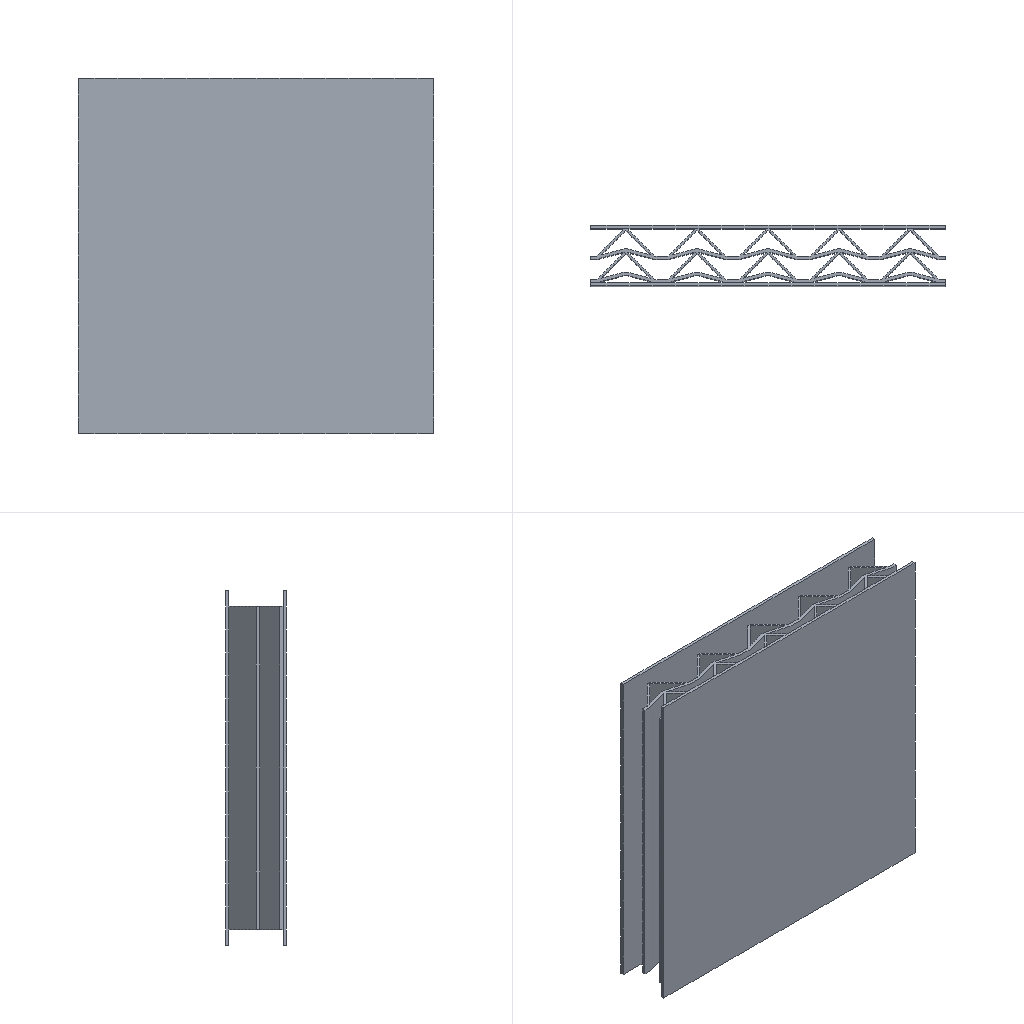Simulation study | abaqus
Set-up summary:
category,name,step,type,value,unit,region
solver,abaqus,,Abaqus/CAE 2024
units,mm-N-s-tonne (MPa),,inferred,E=210000 density=7.85e-09
analysis,Step-1,,dynamic explicit,nlgeom=True; time_period=0.02
mesh,nodes,,,75314
mesh,elements,,,44960
element_type,C3D8R,,,44960
material,Material-2,,E,210000
material,Material-2,,nu,0.3
material,Material-2,,density,7.85e-09
material,PLA,,E,3000
material,PLA,,nu,0.35
material,PLA,,density,1.25e-09
material,PLA,,yield,32
material,PLA,,behaviors,plastic
section,PLA,,solid section,,,Set-1
section,Material-2,,solid section,,,_PickedSet5
section,Material-2,,solid section,,,_PickedSet5
bc,BC-1,initial,encastre,[dofs=ENCASTRE],,_PickedSet18
bc,BC-2,initial,fixed,"[dofs=rx,ry,rz,x,z n=5]",,_PickedSet19
bc,BC-2,Step-1,fixed,"[dofs=rx,ry,rz,x,z n=5]",,_PickedSet19
bc,BC-2,Step-1,displacement,-25 [dofs=y],,_PickedSet19
contact,Int-1,initial,general contact,interaction=IntProp-1; friction=0.15; behavior=hard
constraint,rigid body,,,2
Abaqus input file, long lists of numbers shortened:
*Heading
** Job name: deck Model name: Model-1
** Generated by: Abaqus/CAE 2024
*Preprint, echo=NO, model=NO, history=NO, contact=NO
**
** PARTS
**
*Part, name=P414shuangceng-1
*Node
      1,    56.369,   -16.841,         100.
      2,   53.702,   -16.841,         100.
** (73546 more lines like these left out)
*Element, type=C3D8R
    1,   473,   140,   894,   893,  1381,  1048,  1802,  1801
    2,   894,   735,   342,   893,  1802,  1643,  1250,  1801
** (44158 more lines like these left out)
*Nset, nset=Set-1, generate
     1,  73548,      1
*Elset, elset=Set-1, generate
     1,  44160,      1
** Section: Section-1
*Solid Section, elset=Set-1, material=PLA
,
*End Part
**
*Part, name=P414shuangceng-2
*Node
      1,  -118.298,   16.604,        -110.
      2,  -118.298,   16.604,         -99.
** (880 more lines like these left out)
*Element, type=C3D8R
  1,  43,  44,  65,  64,   1,   2,  23,  22
  2,  44,  45,  66,  65,   2,   3,  24,  23
** (398 more lines like these left out)
*Nset, nset=_PickedSet5, internal, generate
   1,  882,    1
*Elset, elset=_PickedSet5, internal, generate
   1,  400,    1
** Section: Section-2
*Solid Section, elset=_PickedSet5, material=Material-2
,
*End Part
**
*Part, name=P414shuangceng-3
*Node
      1,  -118.298,   -18.841,        -110.
      2,  -118.298,   -18.841,         -99.
** (880 more lines like these left out)
*Element, type=C3D8R
  1,  43,  44,  65,  64,   1,   2,  23,  22
  2,  44,  45,  66,  65,   2,   3,  24,  23
** (398 more lines like these left out)
*Nset, nset=_PickedSet5, internal, generate
   1,  882,    1
*Elset, elset=_PickedSet5, internal, generate
   1,  400,    1
** Section: Section-2
*Solid Section, elset=_PickedSet5, material=Material-2
,
*End Part
**
**
** ASSEMBLY
**
*Assembly, name=Assembly
**
*Instance, name=P414shuangceng-1-1, part=P414shuangceng-1
*End Instance
**
*Instance, name=P414shuangceng-2-1, part=P414shuangceng-2
*End Instance
**
*Instance, name=P414shuangceng-3-1, part=P414shuangceng-3
*End Instance
**
*Node
      1,  -8.298,   18.604, -2.13162821e-14
*Node
      2,  -8.298,   -18.841, -7.10542736e-15
*Nset, nset=Set-5
 1,
*Nset, nset=b_Set-1, instance=P414shuangceng-2-1, generate
   1,  882,    1
*Elset, elset=b_Set-1, instance=P414shuangceng-2-1, generate
   1,  400,    1
*Nset, nset=b_Set-2, instance=P414shuangceng-3-1, generate
   1,  882,    1
*Elset, elset=b_Set-2, instance=P414shuangceng-3-1, generate
   1,  400,    1
*Nset, nset=_PickedSet16, internal
 2,
*Nset, nset=_PickedSet17, internal
 1,
*Nset, nset=_PickedSet18, internal
 2,
*Nset, nset=_PickedSet19, internal
 1,
** Constraint: Constraint-1
*Rigid Body, ref node=_PickedSet16, elset=b_Set-2
** Constraint: Constraint-2
*Rigid Body, ref node=_PickedSet17, elset=b_Set-1
*End Assembly
*Amplitude, name=Amp-1, definition=SMOOTH STEP
             0.,              0.,            0.02,              1.
**
** MATERIALS
**
*Material, name=Material-2
*Density
 7.85e-09,
*Elastic
210000., 0.3
*Material, name=PLA
*Density
 1.25e-09,
*Elastic
3000., 0.35
*Plastic
32.,0.
**
** INTERACTION PROPERTIES
**
*Surface Interaction, name=IntProp-1
*Friction
 0.15,
*Surface Behavior, pressure-overclosure=HARD
**
** BOUNDARY CONDITIONS
**
** Name: BC-1 Type: Symmetry/Antisymmetry/Encastre
*Boundary
_PickedSet18, ENCASTRE
** Name: BC-2 Type: Displacement/Rotation
*Boundary
_PickedSet19, 1, 1
_PickedSet19, 3, 3
_PickedSet19, 4, 4
_PickedSet19, 5, 5
_PickedSet19, 6, 6
**
** INTERACTIONS
**
** Interaction: Int-1
*Contact, op=NEW
*Contact Inclusions, ALL EXTERIOR
*Contact Property Assignment
 ,  , IntProp-1
** ----------------------------------------------------------------
**
** STEP: Step-1
**
*Step, name=Step-1, nlgeom=YES
*Dynamic, Explicit
, 0.02
*Bulk Viscosity
0.06, 1.2
** Mass Scaling: Semi-Automatic
**               Whole Model
*Fixed Mass Scaling, factor=1000.
**
** BOUNDARY CONDITIONS
**
** Name: BC-2 Type: Displacement/Rotation
*Boundary, amplitude=Amp-1
_PickedSet19, 1, 1
_PickedSet19, 2, 2, -25.
_PickedSet19, 3, 3
_PickedSet19, 4, 4
_PickedSet19, 5, 5
_PickedSet19, 6, 6
**
** OUTPUT REQUESTS
**
*Restart, write, number interval=1, time marks=NO
**
** FIELD OUTPUT: F-Output-1
**
*Output, field, time interval=0.01
*Node Output
A, RF, U, V
*Element Output, directions=YES
LE, PE, PEEQ, PEEQVAVG, PEVAVG, S, STATUS, SVAVG
*Contact Output
CSTRESS,
**
** HISTORY OUTPUT: RF
**
*Output, history, time interval=0.01
*Node Output, nset=Set-5
RF1, RF2, RF3, RM1, RM2, RM3, U1, U2
U3, UR1, UR2, UR3
**
** HISTORY OUTPUT: H-Output-1
**
*Output, history, variable=PRESELECT
*End Step
Results summary:
result,odb.job_status,,,JOB_STATUS_COMPLETED_SUCCESSFULLY,"consistent, unstated (Abaqus has no unit system)"
result,steps[0].procedure,Step-1,,"*DYNAMIC, EXPLICIT","consistent, unstated (Abaqus has no unit system)"
result,steps[0].time_period,Step-1,,0.02,"consistent, unstated (Abaqus has no unit system)"
result,steps[0].n_frames,Step-1,,3,"consistent, unstated (Abaqus has no unit system)"
result,steps[0].last_frame.id,Step-1,,2327,"consistent, unstated (Abaqus has no unit system)"
result,steps[0].last_frame.value,Step-1,,0.02,"consistent, unstated (Abaqus has no unit system)"
result,steps[0].last_frame.description,Step-1,,Increment      2327: Step Time =   2.0000E-02,"consistent, unstated (Abaqus has no unit system)"
result,steps[0].completed,Step-1,,True,"consistent, unstated (Abaqus has no unit system)"
result,steps[0].max_U_magnitude,Step-1,,26.091,"consistent, unstated (Abaqus has no unit system)"
result,steps[0].max_S_mises,Step-1,,32.002,"consistent, unstated (Abaqus has no unit system)"
result,steps[0].RF_sum[1],Step-1,,-2087.43,"consistent, unstated (Abaqus has no unit system)"
result,steps[0].RF_sum[2],Step-1,,-18591,"consistent, unstated (Abaqus has no unit system)"
result,steps[0].RF_sum[3],Step-1,,365.496,"consistent, unstated (Abaqus has no unit system)"
result,steps[0].diagnostic.n_increments,Step-1,,21,"consistent, unstated (Abaqus has no unit system)"